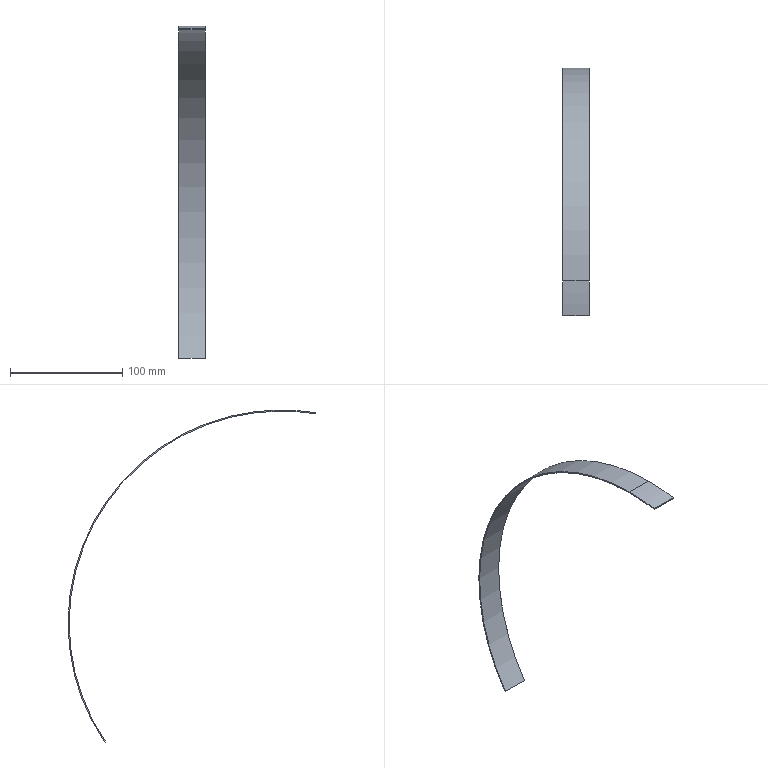Part | STEP file | 09-17 Track inner end plate | 1 solid | 8 faces | box 24 x 221 x 296 mm | volume 10591 mm3 | cylinder 4 | plane 4 | commonest cylinder face diameters 378 x2 380 x2
STEP:
#1=CARTESIAN_POINT('',(0.,0.,0.));
#2=DIRECTION('',(0.,0.,1.));
#3=DIRECTION('',(1.,0.,0.));
#4=AXIS2_PLACEMENT_3D('',#1,#2,#3);
#5=CARTESIAN_POINT('',(0.,156.477,-106.));
#6=VERTEX_POINT('',#5);
#7=CARTESIAN_POINT('',(24.,156.477,-106.));
#8=VERTEX_POINT('',#7);
#9=CARTESIAN_POINT('',(12.,156.477,-106.));
#10=DIRECTION('',(1.,0.,0.));
#11=VECTOR('',#10,1.);
#12=LINE('',#9,#11);
#13=CARTESIAN_POINT('',(24.,0.,0.));
#14=DIRECTION('',(-1.,0.,0.));
#15=DIRECTION('',(0.,0.,1.));
#16=AXIS2_PLACEMENT_3D('',#13,#14,#15);
#17=CYLINDRICAL_SURFACE('',#16,189.);
#18=CARTESIAN_POINT('',(2.166,12.));
#19=DIRECTION('',(0.,-1.));
#20=VECTOR('',#19,1.);
#21=LINE('',#18,#20);
#22=(GEOMETRIC_REPRESENTATION_CONTEXT(2)PARAMETRIC_REPRESENTATION_CONTEXT()REPRESENTATION_CONTEXT('',''));
#23=DEFINITIONAL_REPRESENTATION('',(#21),#22);
#24=PCURVE('',#17,#23);
#25=CARTESIAN_POINT('',(0.,156.477,-106.));
#26=DIRECTION('',(0.,0.,1.));
#27=DIRECTION('',(1.,0.,0.));
#28=AXIS2_PLACEMENT_3D('',#25,#26,#27);
#29=PLANE('',#28);
#30=CARTESIAN_POINT('',(12.,-0.000000036));
#31=DIRECTION('',(1.,0.));
#32=VECTOR('',#31,1.);
#33=LINE('',#30,#32);
#34=(GEOMETRIC_REPRESENTATION_CONTEXT(2)PARAMETRIC_REPRESENTATION_CONTEXT()REPRESENTATION_CONTEXT('',''));
#35=DEFINITIONAL_REPRESENTATION('',(#33),#34);
#36=PCURVE('',#29,#35);
#37=SURFACE_CURVE('',#12,(#24,#36),.PCURVE_S1.);
#38=EDGE_CURVE('',#6,#8,#37,.T.);
#39=ORIENTED_EDGE('',*,*,#38,.F.);
#40=CARTESIAN_POINT('',(0.,0.,189.));
#41=VERTEX_POINT('',#40);
#42=CARTESIAN_POINT('',(0.,0.,0.));
#43=DIRECTION('',(-1.,0.,0.));
#44=DIRECTION('',(0.,0.,1.));
#45=AXIS2_PLACEMENT_3D('',#42,#43,#44);
#46=CIRCLE('',#45,189.);
#47=CARTESIAN_POINT('',(0.,24.));
#48=DIRECTION('',(1.,0.));
#49=VECTOR('',#48,1.);
#50=LINE('',#47,#49);
#51=(GEOMETRIC_REPRESENTATION_CONTEXT(2)PARAMETRIC_REPRESENTATION_CONTEXT()REPRESENTATION_CONTEXT('',''));
#52=DEFINITIONAL_REPRESENTATION('',(#50),#51);
#53=PCURVE('',#17,#52);
#54=CARTESIAN_POINT('',(0.,-31.,191.776));
#55=DIRECTION('',(1.,0.,0.));
#56=DIRECTION('',(0.,0.,-1.));
#57=AXIS2_PLACEMENT_3D('',#54,#55,#56);
#58=PLANE('',#57);
#59=CARTESIAN_POINT('',(2.776,31.));
#60=CARTESIAN_POINT('',(2.776,358.358));
#61=CARTESIAN_POINT('',(286.276,194.679));
#62=CARTESIAN_POINT('',(569.776,31.));
#63=CARTESIAN_POINT('',(286.276,-132.679));
#64=CARTESIAN_POINT('',(2.776,-296.358));
#65=CARTESIAN_POINT('',(2.776,31.));
#66=(BOUNDED_CURVE()B_SPLINE_CURVE(2,(#59,#60,#61,#62,#63,#64,#65),.UNSPECIFIED.,.T.,.F.)B_SPLINE_CURVE_WITH_KNOTS((1,2,2,2,2,1),(-2.094,0.,2.094,4.189,6.283,8.378),.UNSPECIFIED.)CURVE()GEOMETRIC_REPRESENTATION_ITEM()RATIONAL_B_SPLINE_CURVE((1.,0.5,1.,0.5,1.,0.5,1.))REPRESENTATION_ITEM(''));
#67=(GEOMETRIC_REPRESENTATION_CONTEXT(2)PARAMETRIC_REPRESENTATION_CONTEXT()REPRESENTATION_CONTEXT('',''));
#68=DEFINITIONAL_REPRESENTATION('',(#66),#67);
#69=PCURVE('',#58,#68);
#70=SURFACE_CURVE('',#46,(#53,#69),.PCURVE_S1.);
#71=EDGE_CURVE('',#41,#6,#70,.T.);
#72=ORIENTED_EDGE('',*,*,#71,.F.);
#73=CARTESIAN_POINT('',(24.,0.,189.));
#74=VERTEX_POINT('',#73);
#75=CARTESIAN_POINT('',(24.,0.,189.));
#76=DIRECTION('',(-1.,0.,0.));
#77=VECTOR('',#76,1.);
#78=LINE('',#75,#77);
#79=CARTESIAN_POINT('',(0.,0.));
#80=DIRECTION('',(0.,1.));
#81=VECTOR('',#80,1.);
#82=LINE('',#79,#81);
#83=(GEOMETRIC_REPRESENTATION_CONTEXT(2)PARAMETRIC_REPRESENTATION_CONTEXT()REPRESENTATION_CONTEXT('',''));
#84=DEFINITIONAL_REPRESENTATION('',(#82),#83);
#85=PCURVE('',#17,#84);
#86=CARTESIAN_POINT('',(24.,0.,0.));
#87=DIRECTION('',(-1.,0.,0.));
#88=DIRECTION('',(0.,0.,1.));
#89=AXIS2_PLACEMENT_3D('',#86,#87,#88);
#90=CYLINDRICAL_SURFACE('',#89,189.);
#91=CARTESIAN_POINT('',(6.283,0.));
#92=DIRECTION('',(0.,1.));
#93=VECTOR('',#92,1.);
#94=LINE('',#91,#93);
#95=(GEOMETRIC_REPRESENTATION_CONTEXT(2)PARAMETRIC_REPRESENTATION_CONTEXT()REPRESENTATION_CONTEXT('',''));
#96=DEFINITIONAL_REPRESENTATION('',(#94),#95);
#97=PCURVE('',#90,#96);
#98=SURFACE_CURVE('',#78,(#85,#97),.PCURVE_S1.);
#99=EDGE_CURVE('',#74,#41,#98,.T.);
#100=ORIENTED_EDGE('',*,*,#99,.F.);
#101=CARTESIAN_POINT('',(24.,0.,0.));
#102=DIRECTION('',(1.,0.,0.));
#103=DIRECTION('',(0.,0.,1.));
#104=AXIS2_PLACEMENT_3D('',#101,#102,#103);
#105=CIRCLE('',#104,189.);
#106=CARTESIAN_POINT('',(6.283,0.));
#107=DIRECTION('',(-1.,0.));
#108=VECTOR('',#107,1.);
#109=LINE('',#106,#108);
#110=(GEOMETRIC_REPRESENTATION_CONTEXT(2)PARAMETRIC_REPRESENTATION_CONTEXT()REPRESENTATION_CONTEXT('',''));
#111=DEFINITIONAL_REPRESENTATION('',(#109),#110);
#112=PCURVE('',#17,#111);
#113=CARTESIAN_POINT('',(24.,-31.,191.776));
#114=DIRECTION('',(1.,0.,0.));
#115=DIRECTION('',(0.,0.,-1.));
#116=AXIS2_PLACEMENT_3D('',#113,#114,#115);
#117=PLANE('',#116);
#118=CARTESIAN_POINT('',(191.776,31.));
#119=DIRECTION('',(-1.,0.));
#120=AXIS2_PLACEMENT_2D('',#118,#119);
#121=CIRCLE('',#120,189.);
#122=(GEOMETRIC_REPRESENTATION_CONTEXT(2)PARAMETRIC_REPRESENTATION_CONTEXT()REPRESENTATION_CONTEXT('',''));
#123=DEFINITIONAL_REPRESENTATION('',(#121),#122);
#124=PCURVE('',#117,#123);
#125=SURFACE_CURVE('',#105,(#112,#124),.PCURVE_S1.);
#126=EDGE_CURVE('',#8,#74,#125,.T.);
#127=ORIENTED_EDGE('',*,*,#126,.F.);
#128=EDGE_LOOP('',(#39,#72,#100,#127));
#129=FACE_BOUND('',#128,.F.);
#130=ADVANCED_FACE('',(#129),#17,.F.);
#131=CARTESIAN_POINT('',(24.,0.,190.));
#132=VERTEX_POINT('',#131);
#133=CARTESIAN_POINT('',(24.,-31.,187.454));
#134=VERTEX_POINT('',#133);
#135=CARTESIAN_POINT('',(24.,0.,0.));
#136=DIRECTION('',(1.,0.,0.));
#137=DIRECTION('',(0.,0.,1.));
#138=AXIS2_PLACEMENT_3D('',#135,#136,#137);
#139=CIRCLE('',#138,190.);
#140=CARTESIAN_POINT('',(24.,0.,0.));
#141=DIRECTION('',(-1.,0.,0.));
#142=DIRECTION('',(0.,0.,1.));
#143=AXIS2_PLACEMENT_3D('',#140,#141,#142);
#144=CYLINDRICAL_SURFACE('',#143,190.);
#145=CARTESIAN_POINT('',(6.283,0.));
#146=DIRECTION('',(-1.,0.));
#147=VECTOR('',#146,1.);
#148=LINE('',#145,#147);
#149=(GEOMETRIC_REPRESENTATION_CONTEXT(2)PARAMETRIC_REPRESENTATION_CONTEXT()REPRESENTATION_CONTEXT('',''));
#150=DEFINITIONAL_REPRESENTATION('',(#148),#149);
#151=PCURVE('',#144,#150);
#152=CARTESIAN_POINT('',(191.776,31.));
#153=DIRECTION('',(-1.,0.));
#154=AXIS2_PLACEMENT_2D('',#152,#153);
#155=CIRCLE('',#154,190.);
#156=(GEOMETRIC_REPRESENTATION_CONTEXT(2)PARAMETRIC_REPRESENTATION_CONTEXT()REPRESENTATION_CONTEXT('',''));
#157=DEFINITIONAL_REPRESENTATION('',(#155),#156);
#158=PCURVE('',#117,#157);
#159=SURFACE_CURVE('',#139,(#151,#158),.PCURVE_S1.);
#160=EDGE_CURVE('',#132,#134,#159,.T.);
#161=ORIENTED_EDGE('',*,*,#160,.F.);
#162=CARTESIAN_POINT('',(0.,0.,190.));
#163=VERTEX_POINT('',#162);
#164=CARTESIAN_POINT('',(24.,0.,190.));
#165=DIRECTION('',(-1.,0.,0.));
#166=VECTOR('',#165,1.);
#167=LINE('',#164,#166);
#168=CARTESIAN_POINT('',(6.283,0.));
#169=DIRECTION('',(0.,1.));
#170=VECTOR('',#169,1.);
#171=LINE('',#168,#170);
#172=(GEOMETRIC_REPRESENTATION_CONTEXT(2)PARAMETRIC_REPRESENTATION_CONTEXT()REPRESENTATION_CONTEXT('',''));
#173=DEFINITIONAL_REPRESENTATION('',(#171),#172);
#174=PCURVE('',#144,#173);
#175=CARTESIAN_POINT('',(24.,0.,0.));
#176=DIRECTION('',(-1.,0.,0.));
#177=DIRECTION('',(0.,0.,1.));
#178=AXIS2_PLACEMENT_3D('',#175,#176,#177);
#179=CYLINDRICAL_SURFACE('',#178,190.);
#180=CARTESIAN_POINT('',(0.,0.));
#181=DIRECTION('',(0.,1.));
#182=VECTOR('',#181,1.);
#183=LINE('',#180,#182);
#184=(GEOMETRIC_REPRESENTATION_CONTEXT(2)PARAMETRIC_REPRESENTATION_CONTEXT()REPRESENTATION_CONTEXT('',''));
#185=DEFINITIONAL_REPRESENTATION('',(#183),#184);
#186=PCURVE('',#179,#185);
#187=SURFACE_CURVE('',#167,(#174,#186),.PCURVE_S1.);
#188=EDGE_CURVE('',#132,#163,#187,.T.);
#189=ORIENTED_EDGE('',*,*,#188,.T.);
#190=CARTESIAN_POINT('',(0.,-31.,187.454));
#191=VERTEX_POINT('',#190);
#192=CARTESIAN_POINT('',(0.,0.,0.));
#193=DIRECTION('',(1.,0.,0.));
#194=DIRECTION('',(0.,0.,1.));
#195=AXIS2_PLACEMENT_3D('',#192,#193,#194);
#196=CIRCLE('',#195,190.);
#197=CARTESIAN_POINT('',(6.283,24.));
#198=DIRECTION('',(-1.,0.));
#199=VECTOR('',#198,1.);
#200=LINE('',#197,#199);
#201=(GEOMETRIC_REPRESENTATION_CONTEXT(2)PARAMETRIC_REPRESENTATION_CONTEXT()REPRESENTATION_CONTEXT('',''));
#202=DEFINITIONAL_REPRESENTATION('',(#200),#201);
#203=PCURVE('',#144,#202);
#204=CARTESIAN_POINT('',(191.776,31.));
#205=DIRECTION('',(-1.,0.));
#206=AXIS2_PLACEMENT_2D('',#204,#205);
#207=CIRCLE('',#206,190.);
#208=(GEOMETRIC_REPRESENTATION_CONTEXT(2)PARAMETRIC_REPRESENTATION_CONTEXT()REPRESENTATION_CONTEXT('',''));
#209=DEFINITIONAL_REPRESENTATION('',(#207),#208);
#210=PCURVE('',#58,#209);
#211=SURFACE_CURVE('',#196,(#203,#210),.PCURVE_S1.);
#212=EDGE_CURVE('',#163,#191,#211,.T.);
#213=ORIENTED_EDGE('',*,*,#212,.T.);
#214=CARTESIAN_POINT('',(12.,-31.,187.454));
#215=DIRECTION('',(-1.,0.,0.));
#216=VECTOR('',#215,1.);
#217=LINE('',#214,#216);
#218=CARTESIAN_POINT('',(6.119,12.));
#219=DIRECTION('',(0.,1.));
#220=VECTOR('',#219,1.);
#221=LINE('',#218,#220);
#222=(GEOMETRIC_REPRESENTATION_CONTEXT(2)PARAMETRIC_REPRESENTATION_CONTEXT()REPRESENTATION_CONTEXT('',''));
#223=DEFINITIONAL_REPRESENTATION('',(#221),#222);
#224=PCURVE('',#144,#223);
#225=CARTESIAN_POINT('',(0.,-31.,186.44));
#226=DIRECTION('',(0.,1.,0.));
#227=DIRECTION('',(0.,0.,1.));
#228=AXIS2_PLACEMENT_3D('',#225,#226,#227);
#229=PLANE('',#228);
#230=CARTESIAN_POINT('',(1.014,12.));
#231=DIRECTION('',(0.,-1.));
#232=VECTOR('',#231,1.);
#233=LINE('',#230,#232);
#234=(GEOMETRIC_REPRESENTATION_CONTEXT(2)PARAMETRIC_REPRESENTATION_CONTEXT()REPRESENTATION_CONTEXT('',''));
#235=DEFINITIONAL_REPRESENTATION('',(#233),#234);
#236=PCURVE('',#229,#235);
#237=SURFACE_CURVE('',#217,(#224,#236),.PCURVE_S1.);
#238=EDGE_CURVE('',#134,#191,#237,.T.);
#239=ORIENTED_EDGE('',*,*,#238,.F.);
#240=EDGE_LOOP('',(#161,#189,#213,#239));
#241=FACE_BOUND('',#240,.T.);
#242=ADVANCED_FACE('',(#241),#144,.T.);
#243=CARTESIAN_POINT('',(0.,-31.,186.44));
#244=VERTEX_POINT('',#243);
#245=CARTESIAN_POINT('',(0.,0.,0.));
#246=DIRECTION('',(-1.,0.,0.));
#247=DIRECTION('',(0.,0.,1.));
#248=AXIS2_PLACEMENT_3D('',#245,#246,#247);
#249=CIRCLE('',#248,189.);
#250=CARTESIAN_POINT('',(0.,24.));
#251=DIRECTION('',(1.,0.));
#252=VECTOR('',#251,1.);
#253=LINE('',#250,#252);
#254=(GEOMETRIC_REPRESENTATION_CONTEXT(2)PARAMETRIC_REPRESENTATION_CONTEXT()REPRESENTATION_CONTEXT('',''));
#255=DEFINITIONAL_REPRESENTATION('',(#253),#254);
#256=PCURVE('',#90,#255);
#257=CARTESIAN_POINT('',(2.776,31.));
#258=CARTESIAN_POINT('',(2.776,358.358));
#259=CARTESIAN_POINT('',(286.276,194.679));
#260=CARTESIAN_POINT('',(569.776,31.));
#261=CARTESIAN_POINT('',(286.276,-132.679));
#262=CARTESIAN_POINT('',(2.776,-296.358));
#263=CARTESIAN_POINT('',(2.776,31.));
#264=(BOUNDED_CURVE()B_SPLINE_CURVE(2,(#257,#258,#259,#260,#261,#262,#263),.UNSPECIFIED.,.T.,.F.)B_SPLINE_CURVE_WITH_KNOTS((1,2,2,2,2,1),(-2.094,0.,2.094,4.189,6.283,8.378),.UNSPECIFIED.)CURVE()GEOMETRIC_REPRESENTATION_ITEM()RATIONAL_B_SPLINE_CURVE((1.,0.5,1.,0.5,1.,0.5,1.))REPRESENTATION_ITEM(''));
#265=(GEOMETRIC_REPRESENTATION_CONTEXT(2)PARAMETRIC_REPRESENTATION_CONTEXT()REPRESENTATION_CONTEXT('',''));
#266=DEFINITIONAL_REPRESENTATION('',(#264),#265);
#267=PCURVE('',#58,#266);
#268=SURFACE_CURVE('',#249,(#256,#267),.PCURVE_S1.);
#269=EDGE_CURVE('',#244,#41,#268,.T.);
#270=ORIENTED_EDGE('',*,*,#269,.F.);
#271=CARTESIAN_POINT('',(24.,-31.,186.44));
#272=VERTEX_POINT('',#271);
#273=CARTESIAN_POINT('',(12.,-31.,186.44));
#274=DIRECTION('',(-1.,0.,0.));
#275=VECTOR('',#274,1.);
#276=LINE('',#273,#275);
#277=CARTESIAN_POINT('',(6.118,12.));
#278=DIRECTION('',(0.,1.));
#279=VECTOR('',#278,1.);
#280=LINE('',#277,#279);
#281=(GEOMETRIC_REPRESENTATION_CONTEXT(2)PARAMETRIC_REPRESENTATION_CONTEXT()REPRESENTATION_CONTEXT('',''));
#282=DEFINITIONAL_REPRESENTATION('',(#280),#281);
#283=PCURVE('',#90,#282);
#284=CARTESIAN_POINT('',(-0.000000014,12.));
#285=DIRECTION('',(0.,-1.));
#286=VECTOR('',#285,1.);
#287=LINE('',#284,#286);
#288=(GEOMETRIC_REPRESENTATION_CONTEXT(2)PARAMETRIC_REPRESENTATION_CONTEXT()REPRESENTATION_CONTEXT('',''));
#289=DEFINITIONAL_REPRESENTATION('',(#287),#288);
#290=PCURVE('',#229,#289);
#291=SURFACE_CURVE('',#276,(#283,#290),.PCURVE_S1.);
#292=EDGE_CURVE('',#272,#244,#291,.T.);
#293=ORIENTED_EDGE('',*,*,#292,.F.);
#294=CARTESIAN_POINT('',(24.,0.,0.));
#295=DIRECTION('',(1.,0.,0.));
#296=DIRECTION('',(0.,0.,1.));
#297=AXIS2_PLACEMENT_3D('',#294,#295,#296);
#298=CIRCLE('',#297,189.);
#299=CARTESIAN_POINT('',(6.283,0.));
#300=DIRECTION('',(-1.,0.));
#301=VECTOR('',#300,1.);
#302=LINE('',#299,#301);
#303=(GEOMETRIC_REPRESENTATION_CONTEXT(2)PARAMETRIC_REPRESENTATION_CONTEXT()REPRESENTATION_CONTEXT('',''));
#304=DEFINITIONAL_REPRESENTATION('',(#302),#303);
#305=PCURVE('',#90,#304);
#306=CARTESIAN_POINT('',(191.776,31.));
#307=DIRECTION('',(-1.,0.));
#308=AXIS2_PLACEMENT_2D('',#306,#307);
#309=CIRCLE('',#308,189.);
#310=(GEOMETRIC_REPRESENTATION_CONTEXT(2)PARAMETRIC_REPRESENTATION_CONTEXT()REPRESENTATION_CONTEXT('',''));
#311=DEFINITIONAL_REPRESENTATION('',(#309),#310);
#312=PCURVE('',#117,#311);
#313=SURFACE_CURVE('',#298,(#305,#312),.PCURVE_S1.);
#314=EDGE_CURVE('',#74,#272,#313,.T.);
#315=ORIENTED_EDGE('',*,*,#314,.F.);
#316=ORIENTED_EDGE('',*,*,#99,.T.);
#317=EDGE_LOOP('',(#270,#293,#315,#316));
#318=FACE_BOUND('',#317,.F.);
#319=ADVANCED_FACE('',(#318),#90,.F.);
#320=CARTESIAN_POINT('',(24.,157.683,-106.));
#321=VERTEX_POINT('',#320);
#322=CARTESIAN_POINT('',(0.,157.683,-106.));
#323=VERTEX_POINT('',#322);
#324=CARTESIAN_POINT('',(12.,157.683,-106.));
#325=DIRECTION('',(-1.,0.,0.));
#326=VECTOR('',#325,1.);
#327=LINE('',#324,#326);
#328=CARTESIAN_POINT('',(12.,1.206));
#329=DIRECTION('',(-1.,0.));
#330=VECTOR('',#329,1.);
#331=LINE('',#328,#330);
#332=(GEOMETRIC_REPRESENTATION_CONTEXT(2)PARAMETRIC_REPRESENTATION_CONTEXT()REPRESENTATION_CONTEXT('',''));
#333=DEFINITIONAL_REPRESENTATION('',(#331),#332);
#334=PCURVE('',#29,#333);
#335=CARTESIAN_POINT('',(2.163,12.));
#336=DIRECTION('',(0.,1.));
#337=VECTOR('',#336,1.);
#338=LINE('',#335,#337);
#339=(GEOMETRIC_REPRESENTATION_CONTEXT(2)PARAMETRIC_REPRESENTATION_CONTEXT()REPRESENTATION_CONTEXT('',''));
#340=DEFINITIONAL_REPRESENTATION('',(#338),#339);
#341=PCURVE('',#179,#340);
#342=SURFACE_CURVE('',#327,(#334,#341),.PCURVE_S1.);
#343=EDGE_CURVE('',#321,#323,#342,.T.);
#344=ORIENTED_EDGE('',*,*,#343,.F.);
#345=CARTESIAN_POINT('',(24.,157.08,-106.));
#346=DIRECTION('',(0.,1.,0.));
#347=VECTOR('',#346,1.);
#348=LINE('',#345,#347);
#349=CARTESIAN_POINT('',(24.,0.6032));
#350=DIRECTION('',(0.,1.));
#351=VECTOR('',#350,1.);
#352=LINE('',#349,#351);
#353=(GEOMETRIC_REPRESENTATION_CONTEXT(2)PARAMETRIC_REPRESENTATION_CONTEXT()REPRESENTATION_CONTEXT('',''));
#354=DEFINITIONAL_REPRESENTATION('',(#352),#353);
#355=PCURVE('',#29,#354);
#356=CARTESIAN_POINT('',(297.776,188.08));
#357=DIRECTION('',(0.,1.));
#358=VECTOR('',#357,1.);
#359=LINE('',#356,#358);
#360=(GEOMETRIC_REPRESENTATION_CONTEXT(2)PARAMETRIC_REPRESENTATION_CONTEXT()REPRESENTATION_CONTEXT('',''));
#361=DEFINITIONAL_REPRESENTATION('',(#359),#360);
#362=PCURVE('',#117,#361);
#363=SURFACE_CURVE('',#348,(#355,#362),.PCURVE_S1.);
#364=EDGE_CURVE('',#8,#321,#363,.T.);
#365=ORIENTED_EDGE('',*,*,#364,.F.);
#366=ORIENTED_EDGE('',*,*,#38,.F.);
#367=CARTESIAN_POINT('',(0.,157.08,-106.));
#368=DIRECTION('',(0.,-1.,0.));
#369=VECTOR('',#368,1.);
#370=LINE('',#367,#369);
#371=CARTESIAN_POINT('',(0.,0.6032));
#372=DIRECTION('',(0.,-1.));
#373=VECTOR('',#372,1.);
#374=LINE('',#371,#373);
#375=(GEOMETRIC_REPRESENTATION_CONTEXT(2)PARAMETRIC_REPRESENTATION_CONTEXT()REPRESENTATION_CONTEXT('',''));
#376=DEFINITIONAL_REPRESENTATION('',(#374),#375);
#377=PCURVE('',#29,#376);
#378=CARTESIAN_POINT('',(297.776,188.08));
#379=DIRECTION('',(0.,-1.));
#380=VECTOR('',#379,1.);
#381=LINE('',#378,#380);
#382=(GEOMETRIC_REPRESENTATION_CONTEXT(2)PARAMETRIC_REPRESENTATION_CONTEXT()REPRESENTATION_CONTEXT('',''));
#383=DEFINITIONAL_REPRESENTATION('',(#381),#382);
#384=PCURVE('',#58,#383);
#385=SURFACE_CURVE('',#370,(#377,#384),.PCURVE_S1.);
#386=EDGE_CURVE('',#323,#6,#385,.T.);
#387=ORIENTED_EDGE('',*,*,#386,.F.);
#388=EDGE_LOOP('',(#344,#365,#366,#387));
#389=FACE_BOUND('',#388,.T.);
#390=ADVANCED_FACE('',(#389),#29,.F.);
#391=ORIENTED_EDGE('',*,*,#386,.T.);
#392=ORIENTED_EDGE('',*,*,#71,.F.);
#393=ORIENTED_EDGE('',*,*,#269,.F.);
#394=CARTESIAN_POINT('',(0.,-31.,186.947));
#395=DIRECTION('',(0.,0.,1.));
#396=VECTOR('',#395,1.);
#397=LINE('',#394,#396);
#398=CARTESIAN_POINT('',(4.829,0.));
#399=DIRECTION('',(-1.,0.));
#400=VECTOR('',#399,1.);
#401=LINE('',#398,#400);
#402=(GEOMETRIC_REPRESENTATION_CONTEXT(2)PARAMETRIC_REPRESENTATION_CONTEXT()REPRESENTATION_CONTEXT('',''));
#403=DEFINITIONAL_REPRESENTATION('',(#401),#402);
#404=PCURVE('',#58,#403);
#405=CARTESIAN_POINT('',(0.5068,0.));
#406=DIRECTION('',(1.,0.));
#407=VECTOR('',#406,1.);
#408=LINE('',#405,#407);
#409=(GEOMETRIC_REPRESENTATION_CONTEXT(2)PARAMETRIC_REPRESENTATION_CONTEXT()REPRESENTATION_CONTEXT('',''));
#410=DEFINITIONAL_REPRESENTATION('',(#408),#409);
#411=PCURVE('',#229,#410);
#412=SURFACE_CURVE('',#397,(#404,#411),.PCURVE_S1.);
#413=EDGE_CURVE('',#244,#191,#412,.T.);
#414=ORIENTED_EDGE('',*,*,#413,.T.);
#415=ORIENTED_EDGE('',*,*,#212,.F.);
#416=CARTESIAN_POINT('',(0.,0.,0.));
#417=DIRECTION('',(1.,0.,0.));
#418=DIRECTION('',(0.,0.,1.));
#419=AXIS2_PLACEMENT_3D('',#416,#417,#418);
#420=CIRCLE('',#419,190.);
#421=CARTESIAN_POINT('',(191.776,31.));
#422=DIRECTION('',(-1.,0.));
#423=AXIS2_PLACEMENT_2D('',#421,#422);
#424=CIRCLE('',#423,190.);
#425=(GEOMETRIC_REPRESENTATION_CONTEXT(2)PARAMETRIC_REPRESENTATION_CONTEXT()REPRESENTATION_CONTEXT('',''));
#426=DEFINITIONAL_REPRESENTATION('',(#424),#425);
#427=PCURVE('',#58,#426);
#428=CARTESIAN_POINT('',(6.283,24.));
#429=DIRECTION('',(-1.,0.));
#430=VECTOR('',#429,1.);
#431=LINE('',#428,#430);
#432=(GEOMETRIC_REPRESENTATION_CONTEXT(2)PARAMETRIC_REPRESENTATION_CONTEXT()REPRESENTATION_CONTEXT('',''));
#433=DEFINITIONAL_REPRESENTATION('',(#431),#432);
#434=PCURVE('',#179,#433);
#435=SURFACE_CURVE('',#420,(#427,#434),.PCURVE_S1.);
#436=EDGE_CURVE('',#323,#163,#435,.T.);
#437=ORIENTED_EDGE('',*,*,#436,.F.);
#438=EDGE_LOOP('',(#391,#392,#393,#414,#415,#437));
#439=FACE_BOUND('',#438,.T.);
#440=ADVANCED_FACE('',(#439),#58,.F.);
#441=ORIENTED_EDGE('',*,*,#126,.F.);
#442=ORIENTED_EDGE('',*,*,#364,.T.);
#443=CARTESIAN_POINT('',(24.,0.,0.));
#444=DIRECTION('',(1.,0.,0.));
#445=DIRECTION('',(0.,0.,1.));
#446=AXIS2_PLACEMENT_3D('',#443,#444,#445);
#447=CIRCLE('',#446,190.);
#448=CARTESIAN_POINT('',(191.776,31.));
#449=DIRECTION('',(-1.,0.));
#450=AXIS2_PLACEMENT_2D('',#448,#449);
#451=CIRCLE('',#450,190.);
#452=(GEOMETRIC_REPRESENTATION_CONTEXT(2)PARAMETRIC_REPRESENTATION_CONTEXT()REPRESENTATION_CONTEXT('',''));
#453=DEFINITIONAL_REPRESENTATION('',(#451),#452);
#454=PCURVE('',#117,#453);
#455=CARTESIAN_POINT('',(6.283,0.));
#456=DIRECTION('',(-1.,0.));
#457=VECTOR('',#456,1.);
#458=LINE('',#455,#457);
#459=(GEOMETRIC_REPRESENTATION_CONTEXT(2)PARAMETRIC_REPRESENTATION_CONTEXT()REPRESENTATION_CONTEXT('',''));
#460=DEFINITIONAL_REPRESENTATION('',(#458),#459);
#461=PCURVE('',#179,#460);
#462=SURFACE_CURVE('',#447,(#454,#461),.PCURVE_S1.);
#463=EDGE_CURVE('',#321,#132,#462,.T.);
#464=ORIENTED_EDGE('',*,*,#463,.T.);
#465=ORIENTED_EDGE('',*,*,#160,.T.);
#466=CARTESIAN_POINT('',(24.,-31.,42.888));
#467=DIRECTION('',(0.,0.,-1.));
#468=VECTOR('',#467,1.);
#469=LINE('',#466,#468);
#470=CARTESIAN_POINT('',(148.888,0.));
#471=DIRECTION('',(1.,0.));
#472=VECTOR('',#471,1.);
#473=LINE('',#470,#472);
#474=(GEOMETRIC_REPRESENTATION_CONTEXT(2)PARAMETRIC_REPRESENTATION_CONTEXT()REPRESENTATION_CONTEXT('',''));
#475=DEFINITIONAL_REPRESENTATION('',(#473),#474);
#476=PCURVE('',#117,#475);
#477=CARTESIAN_POINT('',(-143.552,24.));
#478=DIRECTION('',(-1.,0.));
#479=VECTOR('',#478,1.);
#480=LINE('',#477,#479);
#481=(GEOMETRIC_REPRESENTATION_CONTEXT(2)PARAMETRIC_REPRESENTATION_CONTEXT()REPRESENTATION_CONTEXT('',''));
#482=DEFINITIONAL_REPRESENTATION('',(#480),#481);
#483=PCURVE('',#229,#482);
#484=SURFACE_CURVE('',#469,(#476,#483),.PCURVE_S1.);
#485=EDGE_CURVE('',#134,#272,#484,.T.);
#486=ORIENTED_EDGE('',*,*,#485,.T.);
#487=ORIENTED_EDGE('',*,*,#314,.F.);
#488=EDGE_LOOP('',(#441,#442,#464,#465,#486,#487));
#489=FACE_BOUND('',#488,.T.);
#490=ADVANCED_FACE('',(#489),#117,.T.);
#491=ORIENTED_EDGE('',*,*,#188,.F.);
#492=ORIENTED_EDGE('',*,*,#463,.F.);
#493=ORIENTED_EDGE('',*,*,#343,.T.);
#494=ORIENTED_EDGE('',*,*,#436,.T.);
#495=EDGE_LOOP('',(#491,#492,#493,#494));
#496=FACE_BOUND('',#495,.T.);
#497=ADVANCED_FACE('',(#496),#179,.T.);
#498=ORIENTED_EDGE('',*,*,#292,.F.);
#499=ORIENTED_EDGE('',*,*,#485,.F.);
#500=ORIENTED_EDGE('',*,*,#238,.T.);
#501=ORIENTED_EDGE('',*,*,#413,.F.);
#502=EDGE_LOOP('',(#498,#499,#500,#501));
#503=FACE_BOUND('',#502,.T.);
#504=ADVANCED_FACE('',(#503),#229,.F.);
#505=CLOSED_SHELL('',(#130,#242,#319,#390,#440,#490,#497,#504));
#506=MANIFOLD_SOLID_BREP('',#505);
#507=(LENGTH_UNIT()NAMED_UNIT(*)SI_UNIT(.MILLI.,.METRE.));
#508=UNCERTAINTY_MEASURE_WITH_UNIT(LENGTH_MEASURE(0.0000001),#507,'','');
#509=(NAMED_UNIT(*)PLANE_ANGLE_UNIT()SI_UNIT($,.RADIAN.));
#510=(NAMED_UNIT(*)SI_UNIT($,.STERADIAN.)SOLID_ANGLE_UNIT());
#511=(GEOMETRIC_REPRESENTATION_CONTEXT(3)GLOBAL_UNCERTAINTY_ASSIGNED_CONTEXT((#508))GLOBAL_UNIT_ASSIGNED_CONTEXT((#507,#509,#510))REPRESENTATION_CONTEXT('',''));
#512=ADVANCED_BREP_SHAPE_REPRESENTATION('',(#4,#506),#511);